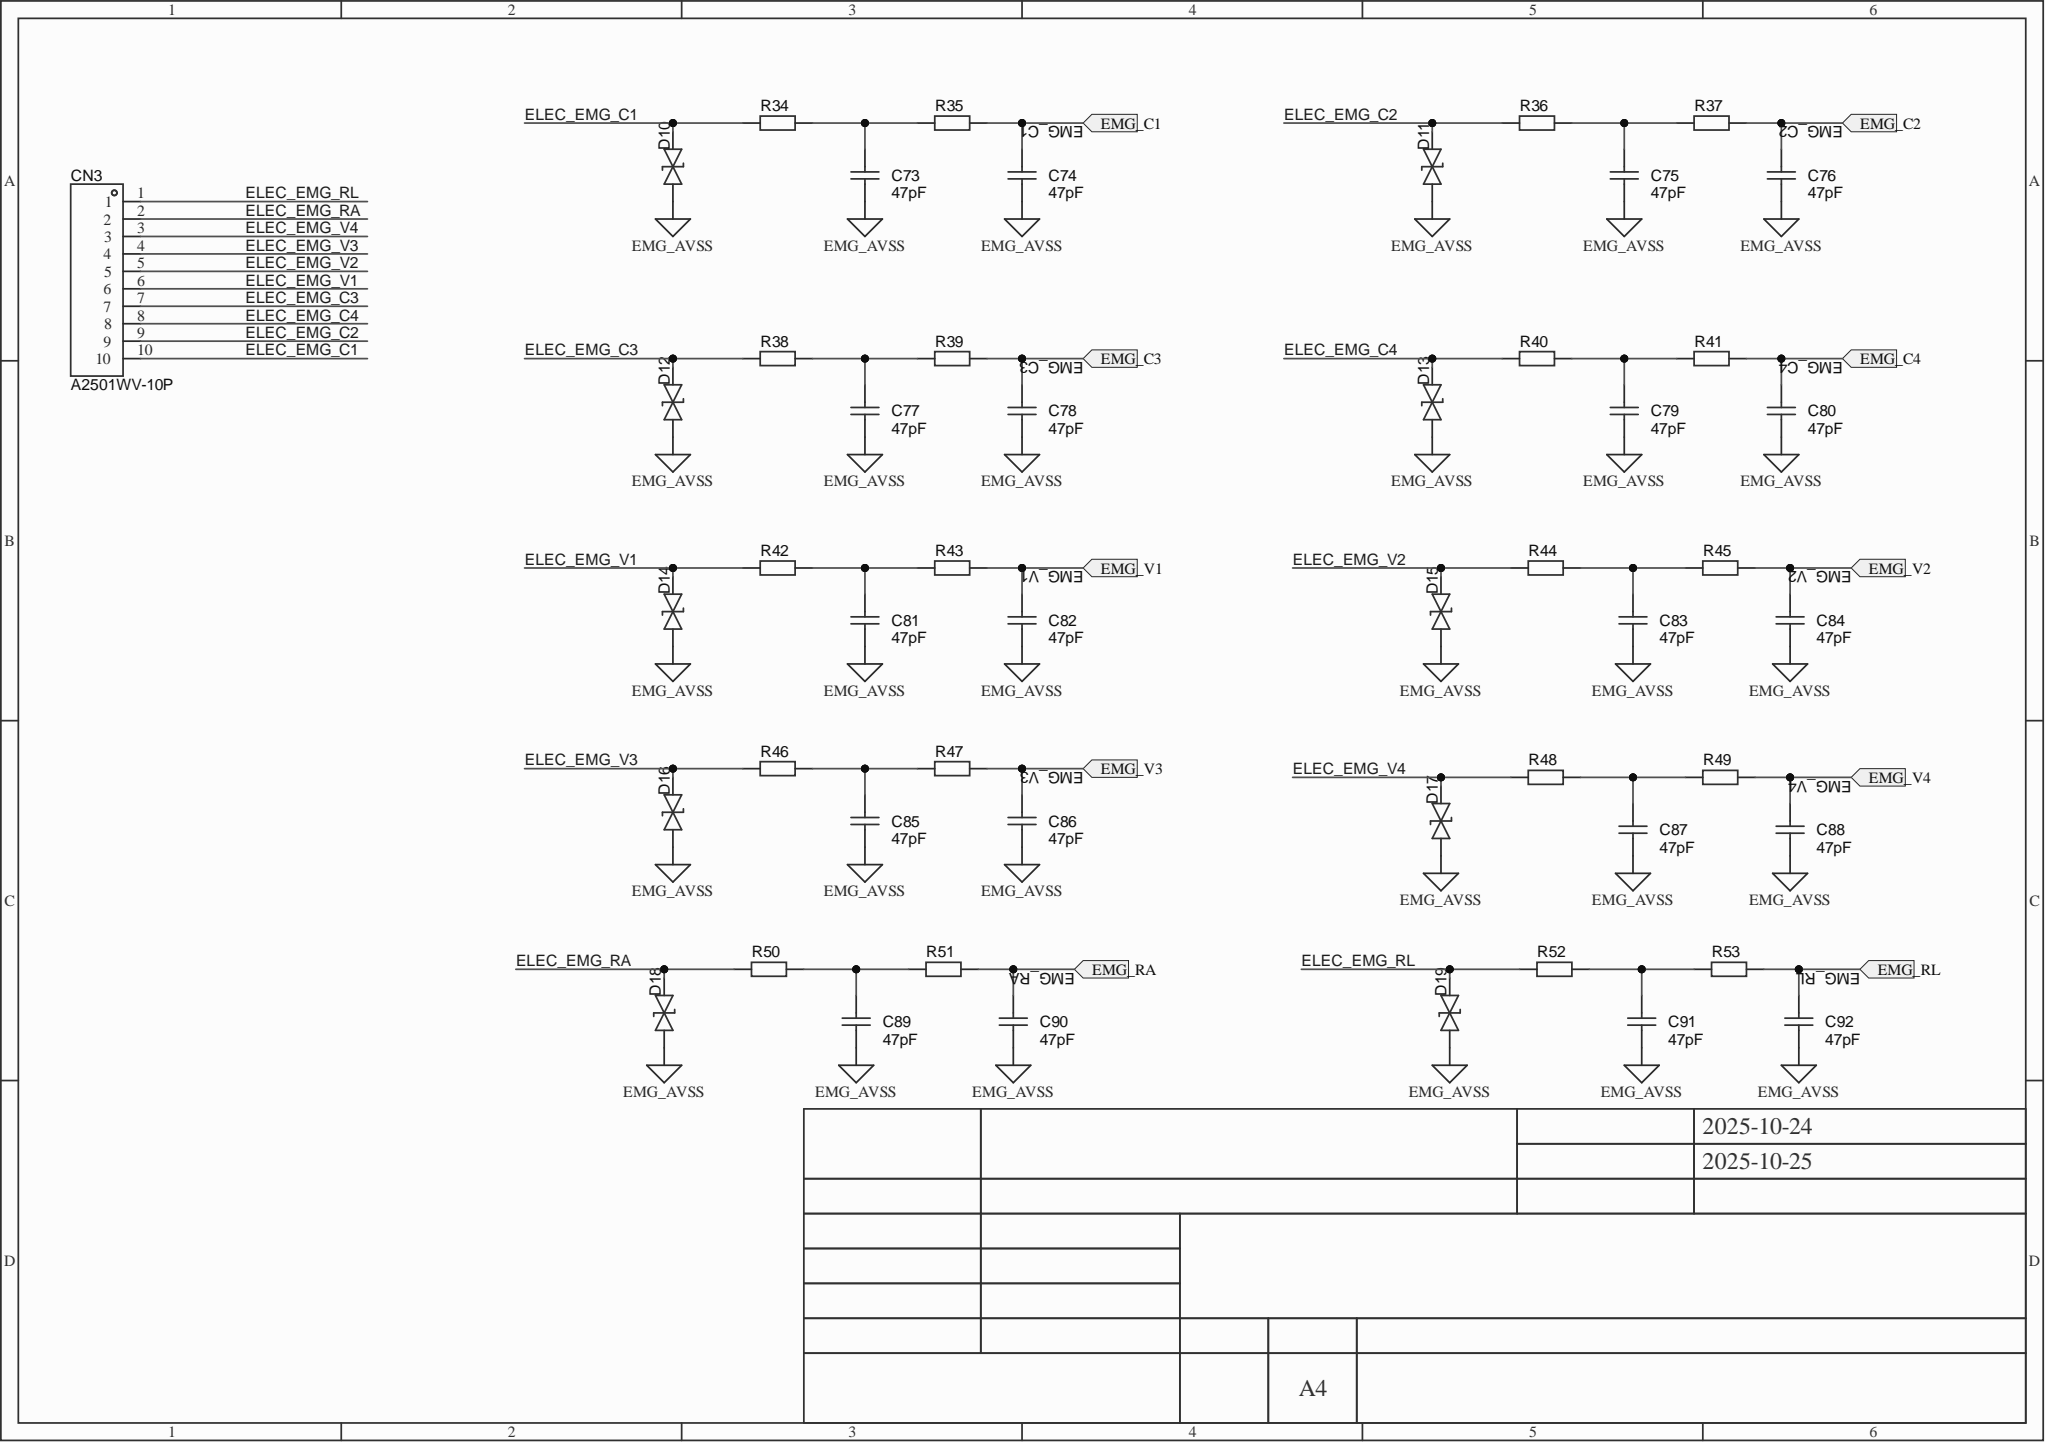Circuit board | Altium Designer | 211 parts | 126 nets | one sheet of the schematic
Parts on this sheet (reference | value | footprint):
C73 | 47pF | C0402
C74 | 47pF | C0402
C75 | 47pF | C0402
C76 | 47pF | C0402
C77 | 47pF | C0402
C78 | 47pF | C0402
C79 | 47pF | C0402
C80 | 47pF | C0402
C81 | 47pF | C0402
C82 | 47pF | C0402
C83 | 47pF | C0402
C84 | 47pF | C0402
C85 | 47pF | C0402
C86 | 47pF | C0402
C87 | 47pF | C0402
C88 | 47pF | C0402
C89 | 47pF | C0402
C90 | 47pF | C0402
C91 | 47pF | C0402
C92 | 47pF | C0402
CN3 | A2501WV-10P | CONN-TH_A2501WV-10P
D10 | TPD1E10B06DPYR-TP | X1-DFN1006-2_L1.0-W0.6-BI
D11 | TPD1E10B06DPYR-TP | X1-DFN1006-2_L1.0-W0.6-BI
D12 | TPD1E10B06DPYR-TP | X1-DFN1006-2_L1.0-W0.6-BI
D13 | TPD1E10B06DPYR-TP | X1-DFN1006-2_L1.0-W0.6-BI
D14 | TPD1E10B06DPYR-TP | X1-DFN1006-2_L1.0-W0.6-BI
D15 | TPD1E10B06DPYR-TP | X1-DFN1006-2_L1.0-W0.6-BI
D16 | TPD1E10B06DPYR-TP | X1-DFN1006-2_L1.0-W0.6-BI
D17 | TPD1E10B06DPYR-TP | X1-DFN1006-2_L1.0-W0.6-BI
D18 | TPD1E10B06DPYR-TP | X1-DFN1006-2_L1.0-W0.6-BI
D19 | TPD1E10B06DPYR-TP | X1-DFN1006-2_L1.0-W0.6-BI
R34 | R0402
R35 | R0402
R36 | R0402
R37 | R0402
R38 | R0402
R39 | R0402
R40 | R0402
R41 | R0402
R42 | R0402
R43 | R0402
R44 | R0402
R45 | R0402
R46 | R0402
R47 | R0402
R48 | R0402
R49 | R0402
R50 | R0402
R51 | R0402
R52 | R0402
R53 | R0402
Nets of these parts (net: part-pin ...):
NetC91_2: C91-2 R52-2 R53-1
NetC89_2: C89-2 R50-2 R51-1
NetC87_2: C87-2 R48-2 R49-1
NetC85_2: C85-2 R46-2 R47-1
NetC83_2: C83-2 R44-2 R45-1
NetC81_2: C81-2 R42-2 R43-1
NetC79_2: C79-2 R40-2 R41-1
NetC77_2: C77-2 R38-2 R39-1
NetC75_2: C75-2 R36-2 R37-1
NetC73_2: C73-2 R34-2 R35-1
EMG_V4: C88-2 R49-2
EMG_V3: C86-2 R47-2
EMG_V2: C84-2 R45-2
EMG_V1: C82-2 R43-2
EMG_RL: C92-2 R53-2
EMG_RA: C90-2 R51-2
EMG_C4: C80-2 R41-2
EMG_C3: C78-2 R39-2
EMG_C2: C76-2 R37-2
EMG_C1: C74-2 R35-2
EMG_AVSS1: C73-1 C74-1 C75-1 C76-1 C77-1 C78-1 C79-1 C80-1 C81-1 C82-1 C83-1 C84-1 C85-1 C86-1 C87-1 C88-1 C89-1 C90-1 C91-1 C92-1 D10-1 D11-1 D12-1 D13-1 D14-1 D15-1 D16-1 D17-1 D18-1 D19-1
ELEC_EMG_V4: CN3-3 D17-2 R48-1
ELEC_EMG_V3: CN3-4 D16-2 R46-1
ELEC_EMG_V2: CN3-5 D15-2 R44-1
ELEC_EMG_V1: CN3-6 D14-2 R42-1
ELEC_EMG_RL: CN3-1 D19-2 R52-1
ELEC_EMG_RA: CN3-2 D18-2 R50-1
ELEC_EMG_C4: CN3-8 D13-2 R40-1
ELEC_EMG_C3: CN3-7 D12-2 R38-1
ELEC_EMG_C2: CN3-9 D11-2 R36-1
ELEC_EMG_C1: CN3-10 D10-2 R34-1